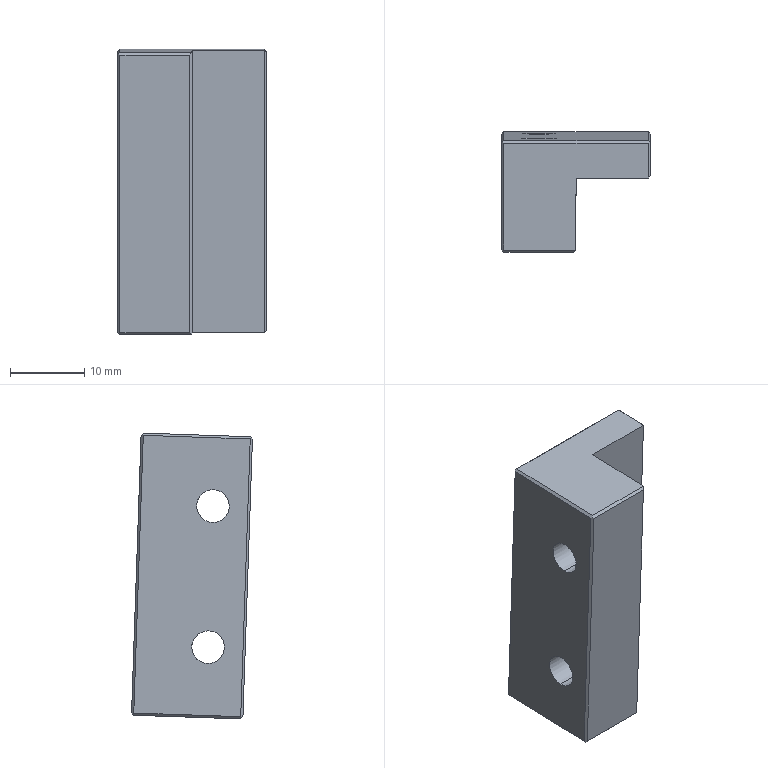Part | NX | 1 solid | 41 faces | box 20 x 16.27 x 38.47 mm | volume 7135 mm3 | plane 21 | cylinder 12 | cone 8 | commonest cylinder face diameters 3.3 x8 4.4 x4